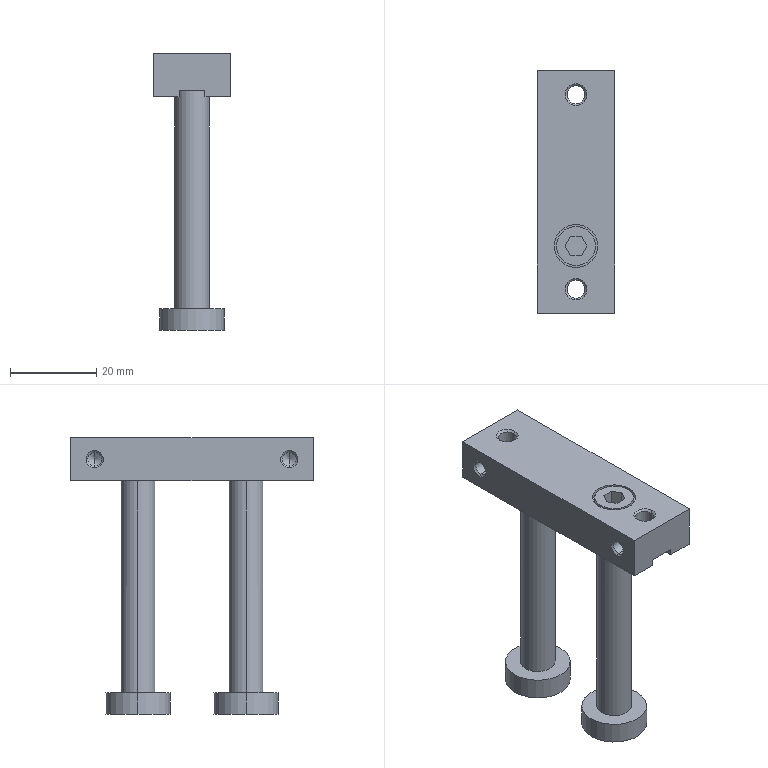Part | SolidWorks | features ICE 5, HoleWzd 4, RefAxis 3, RevCut 2, Revolution 2, 3DProfileFeature 1, Extrusion 1 | 1 solid | 90 faces | box 18 x 56 x 64 mm | volume 15836 mm3 | plane 38 | cylinder 28 | cone 24 | commonest cylinder face diameters 3.242 x8 4.134 x4 8 x4 15 x4 5 x2 6 x2